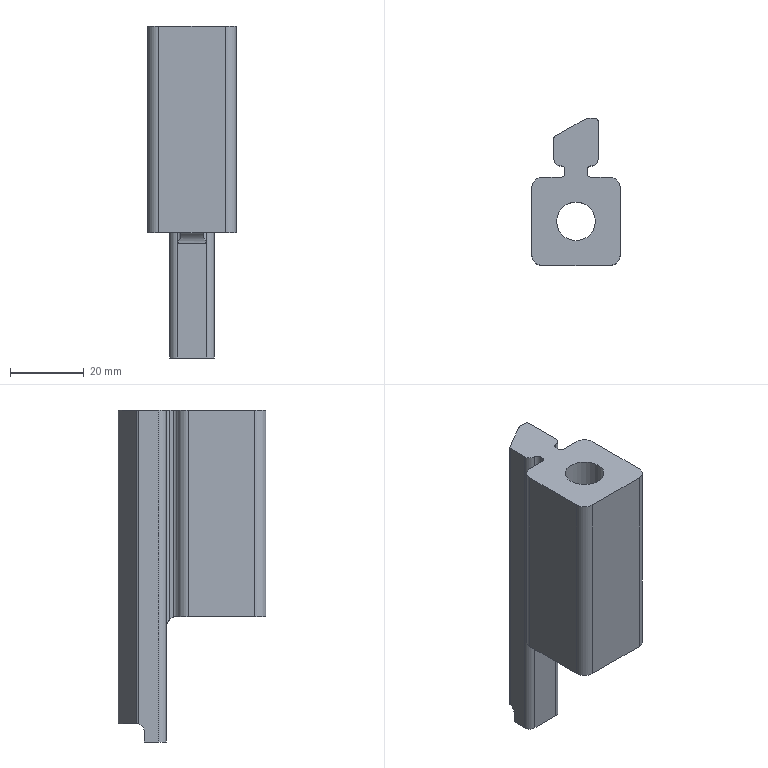Part | STEP file | gslz 2016.10.28-10_id54_x_t | 1 solid | 35 faces | box 24 x 40 x 90 mm | volume 34487 mm3 | plane 18 | cylinder 17 | commonest cylinder face diameters 2 x5 6 x5 4 x4 1 x1 10.5 x1 17 x1